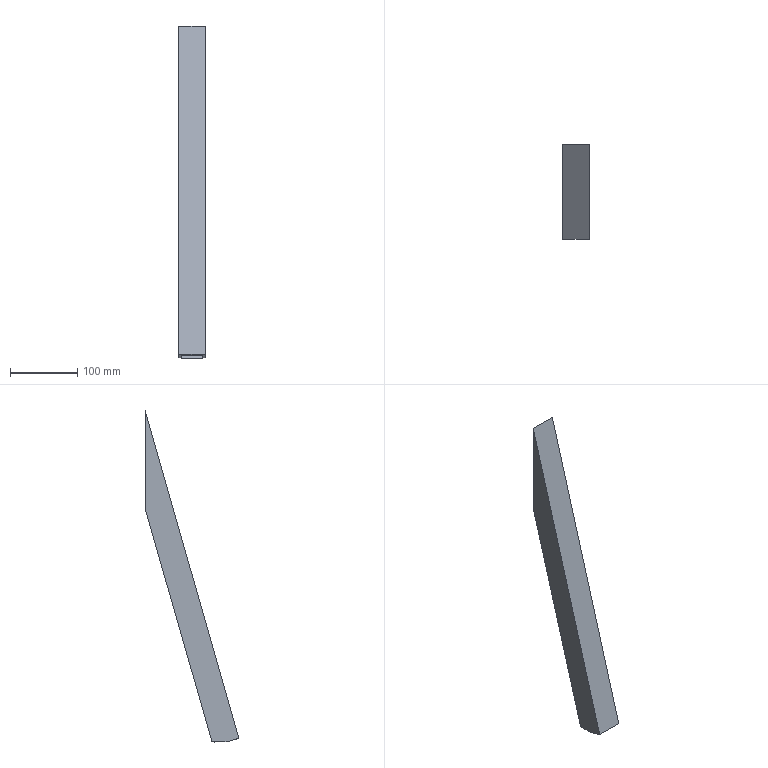Part | SolidWorks | features BaseBody 1 | 1 solid | 11 faces | box 40 x 139.228 x 491.982 mm | volume 250092 mm3 | plane 11
STEP:
#1=CARTESIAN_POINT('',(-230.,-189.228,31.503));
#2=VERTEX_POINT('',#1);
#3=CARTESIAN_POINT('',(-230.,-50.,517.982));
#4=VERTEX_POINT('',#3);
#5=CARTESIAN_POINT('',(-230.,-189.228,31.503));
#6=DIRECTION('',(0.,0.2751,0.9614));
#7=VECTOR('',#6,1000.);
#8=LINE('',#5,#7);
#9=EDGE_CURVE('',#2,#4,#8,.T.);
#10=ORIENTED_EDGE('',*,*,#9,.F.);
#11=CARTESIAN_POINT('',(-190.,-189.228,31.503));
#12=VERTEX_POINT('',#11);
#13=CARTESIAN_POINT('',(-190.,-189.228,31.503));
#14=DIRECTION('',(-1.,0.,0.));
#15=VECTOR('',#14,1000.);
#16=LINE('',#13,#15);
#17=EDGE_CURVE('',#12,#2,#16,.T.);
#18=ORIENTED_EDGE('',*,*,#17,.F.);
#19=CARTESIAN_POINT('',(-190.,-50.,517.982));
#20=VERTEX_POINT('',#19);
#21=CARTESIAN_POINT('',(-190.,-189.228,31.503));
#22=DIRECTION('',(0.,-0.2751,-0.9614));
#23=VECTOR('',#22,1000.);
#24=LINE('',#21,#23);
#25=EDGE_CURVE('',#20,#12,#24,.T.);
#26=ORIENTED_EDGE('',*,*,#25,.F.);
#27=CARTESIAN_POINT('',(-190.,-50.,517.982));
#28=DIRECTION('',(1.,0.,0.));
#29=VECTOR('',#28,1000.);
#30=LINE('',#27,#29);
#31=EDGE_CURVE('',#4,#20,#30,.T.);
#32=ORIENTED_EDGE('',*,*,#31,.F.);
#33=EDGE_LOOP('',(#10,#18,#26,#32));
#34=FACE_OUTER_BOUND('',#33,.T.);
#35=CARTESIAN_POINT('',(-190.,-189.228,31.503));
#36=DIRECTION('',(0.,0.9614,-0.2751));
#37=DIRECTION('',(0.,0.2751,0.9614));
#38=AXIS2_PLACEMENT_3D('',#35,#36,#37);
#39=PLANE('',#38);
#40=ADVANCED_FACE('',(#34),#39,.F.);
#41=CARTESIAN_POINT('',(-226.,-50.,503.445));
#42=VERTEX_POINT('',#41);
#43=CARTESIAN_POINT('',(-226.,-50.,387.144));
#44=VERTEX_POINT('',#43);
#45=CARTESIAN_POINT('',(-226.,-50.,28.));
#46=DIRECTION('',(0.,0.,-1.));
#47=VECTOR('',#46,1000.);
#48=LINE('',#45,#47);
#49=EDGE_CURVE('',#42,#44,#48,.T.);
#50=ORIENTED_EDGE('',*,*,#49,.T.);
#51=CARTESIAN_POINT('',(-194.,-50.,387.144));
#52=VERTEX_POINT('',#51);
#53=CARTESIAN_POINT('',(-260.,-50.,387.144));
#54=DIRECTION('',(1.,0.,0.));
#55=VECTOR('',#54,1000.);
#56=LINE('',#53,#55);
#57=EDGE_CURVE('',#44,#52,#56,.T.);
#58=ORIENTED_EDGE('',*,*,#57,.T.);
#59=CARTESIAN_POINT('',(-194.,-50.,503.445));
#60=VERTEX_POINT('',#59);
#61=CARTESIAN_POINT('',(-194.,-50.,28.));
#62=DIRECTION('',(0.,0.,1.));
#63=VECTOR('',#62,1000.);
#64=LINE('',#61,#63);
#65=EDGE_CURVE('',#52,#60,#64,.T.);
#66=ORIENTED_EDGE('',*,*,#65,.T.);
#67=CARTESIAN_POINT('',(-260.,-50.,503.445));
#68=DIRECTION('',(-1.,0.,0.));
#69=VECTOR('',#68,1000.);
#70=LINE('',#67,#69);
#71=EDGE_CURVE('',#60,#42,#70,.T.);
#72=ORIENTED_EDGE('',*,*,#71,.T.);
#73=EDGE_LOOP('',(#50,#58,#66,#72));
#74=FACE_BOUND('',#73,.T.);
#75=CARTESIAN_POINT('',(-190.,-50.,372.606));
#76=VERTEX_POINT('',#75);
#77=CARTESIAN_POINT('',(-190.,-50.,28.));
#78=DIRECTION('',(0.,0.,-1.));
#79=VECTOR('',#78,1000.);
#80=LINE('',#77,#79);
#81=EDGE_CURVE('',#20,#76,#80,.T.);
#82=ORIENTED_EDGE('',*,*,#81,.T.);
#83=CARTESIAN_POINT('',(-230.,-50.,372.606));
#84=VERTEX_POINT('',#83);
#85=CARTESIAN_POINT('',(-260.,-50.,372.606));
#86=DIRECTION('',(-1.,0.,0.));
#87=VECTOR('',#86,1000.);
#88=LINE('',#85,#87);
#89=EDGE_CURVE('',#76,#84,#88,.T.);
#90=ORIENTED_EDGE('',*,*,#89,.T.);
#91=CARTESIAN_POINT('',(-230.,-50.,28.));
#92=DIRECTION('',(0.,0.,1.));
#93=VECTOR('',#92,1000.);
#94=LINE('',#91,#93);
#95=EDGE_CURVE('',#84,#4,#94,.T.);
#96=ORIENTED_EDGE('',*,*,#95,.T.);
#97=ORIENTED_EDGE('',*,*,#31,.T.);
#98=EDGE_LOOP('',(#82,#90,#96,#97));
#99=FACE_OUTER_BOUND('',#98,.T.);
#100=CARTESIAN_POINT('',(-260.,-50.,28.));
#101=DIRECTION('',(0.,1.,0.));
#102=DIRECTION('',(0.,0.,1.));
#103=AXIS2_PLACEMENT_3D('',#100,#101,#102);
#104=PLANE('',#103);
#105=ADVANCED_FACE('',(#74,#99),#104,.T.);
#106=ORIENTED_EDGE('',*,*,#9,.T.);
#107=ORIENTED_EDGE('',*,*,#95,.F.);
#108=CARTESIAN_POINT('',(-230.,-149.197,26.));
#109=VERTEX_POINT('',#108);
#110=CARTESIAN_POINT('',(-230.,-50.,372.606));
#111=DIRECTION('',(0.,-0.2751,-0.9614));
#112=VECTOR('',#111,1000.);
#113=LINE('',#110,#112);
#114=EDGE_CURVE('',#84,#109,#113,.T.);
#115=ORIENTED_EDGE('',*,*,#114,.T.);
#116=CARTESIAN_POINT('',(-230.,-170.,26.));
#117=VERTEX_POINT('',#116);
#118=CARTESIAN_POINT('',(-230.,-189.228,26.));
#119=DIRECTION('',(0.,-1.,0.));
#120=VECTOR('',#119,1000.);
#121=LINE('',#118,#120);
#122=EDGE_CURVE('',#109,#117,#121,.T.);
#123=ORIENTED_EDGE('',*,*,#122,.T.);
#124=CARTESIAN_POINT('',(-230.,-170.,26.));
#125=DIRECTION('',(0.,-0.9614,0.2751));
#126=VECTOR('',#125,1000.);
#127=LINE('',#124,#126);
#128=EDGE_CURVE('',#117,#2,#127,.T.);
#129=ORIENTED_EDGE('',*,*,#128,.T.);
#130=EDGE_LOOP('',(#106,#107,#115,#123,#129));
#131=FACE_OUTER_BOUND('',#130,.T.);
#132=CARTESIAN_POINT('',(-230.,-189.228,31.503));
#133=DIRECTION('',(-1.,0.,0.));
#134=DIRECTION('',(0.,0.,1.));
#135=AXIS2_PLACEMENT_3D('',#132,#133,#134);
#136=PLANE('',#135);
#137=ADVANCED_FACE('',(#131),#136,.T.);
#138=CARTESIAN_POINT('',(-226.,-185.382,30.402));
#139=VERTEX_POINT('',#138);
#140=CARTESIAN_POINT('',(-226.,-170.,26.));
#141=VERTEX_POINT('',#140);
#142=CARTESIAN_POINT('',(-226.,-189.228,31.503));
#143=DIRECTION('',(0.,0.9614,-0.2751));
#144=VECTOR('',#143,1000.);
#145=LINE('',#142,#144);
#146=EDGE_CURVE('',#139,#141,#145,.T.);
#147=ORIENTED_EDGE('',*,*,#146,.F.);
#148=CARTESIAN_POINT('',(-194.,-185.382,30.402));
#149=VERTEX_POINT('',#148);
#150=CARTESIAN_POINT('',(-190.,-185.382,30.402));
#151=DIRECTION('',(-1.,0.,0.));
#152=VECTOR('',#151,1000.);
#153=LINE('',#150,#152);
#154=EDGE_CURVE('',#149,#139,#153,.T.);
#155=ORIENTED_EDGE('',*,*,#154,.F.);
#156=CARTESIAN_POINT('',(-194.,-170.,26.));
#157=VERTEX_POINT('',#156);
#158=CARTESIAN_POINT('',(-194.,-189.228,31.503));
#159=DIRECTION('',(0.,-0.9614,0.2751));
#160=VECTOR('',#159,1000.);
#161=LINE('',#158,#160);
#162=EDGE_CURVE('',#157,#149,#161,.T.);
#163=ORIENTED_EDGE('',*,*,#162,.F.);
#164=CARTESIAN_POINT('',(-190.,-170.,26.));
#165=VERTEX_POINT('',#164);
#166=CARTESIAN_POINT('',(-190.,-170.,26.));
#167=DIRECTION('',(-1.,0.,0.));
#168=VECTOR('',#167,1000.);
#169=LINE('',#166,#168);
#170=EDGE_CURVE('',#165,#157,#169,.T.);
#171=ORIENTED_EDGE('',*,*,#170,.F.);
#172=CARTESIAN_POINT('',(-190.,-189.228,31.503));
#173=DIRECTION('',(0.,0.9614,-0.2751));
#174=VECTOR('',#173,1000.);
#175=LINE('',#172,#174);
#176=EDGE_CURVE('',#12,#165,#175,.T.);
#177=ORIENTED_EDGE('',*,*,#176,.F.);
#178=ORIENTED_EDGE('',*,*,#17,.T.);
#179=ORIENTED_EDGE('',*,*,#128,.F.);
#180=CARTESIAN_POINT('',(-190.,-170.,26.));
#181=DIRECTION('',(-1.,0.,0.));
#182=VECTOR('',#181,1000.);
#183=LINE('',#180,#182);
#184=EDGE_CURVE('',#141,#117,#183,.T.);
#185=ORIENTED_EDGE('',*,*,#184,.F.);
#186=EDGE_LOOP('',(#147,#155,#163,#171,#177,#178,#179,#185));
#187=FACE_OUTER_BOUND('',#186,.T.);
#188=CARTESIAN_POINT('',(-190.,-189.228,31.503));
#189=DIRECTION('',(0.,0.2751,0.9614));
#190=DIRECTION('',(0.,-0.9614,0.2751));
#191=AXIS2_PLACEMENT_3D('',#188,#189,#190);
#192=PLANE('',#191);
#193=ADVANCED_FACE('',(#187),#192,.F.);
#194=ORIENTED_EDGE('',*,*,#25,.T.);
#195=ORIENTED_EDGE('',*,*,#176,.T.);
#196=CARTESIAN_POINT('',(-190.,-149.197,26.));
#197=VERTEX_POINT('',#196);
#198=CARTESIAN_POINT('',(-190.,-189.228,26.));
#199=DIRECTION('',(0.,-1.,0.));
#200=VECTOR('',#199,1000.);
#201=LINE('',#198,#200);
#202=EDGE_CURVE('',#197,#165,#201,.T.);
#203=ORIENTED_EDGE('',*,*,#202,.F.);
#204=CARTESIAN_POINT('',(-190.,-50.,372.606));
#205=DIRECTION('',(0.,-0.2751,-0.9614));
#206=VECTOR('',#205,1000.);
#207=LINE('',#204,#206);
#208=EDGE_CURVE('',#76,#197,#207,.T.);
#209=ORIENTED_EDGE('',*,*,#208,.F.);
#210=ORIENTED_EDGE('',*,*,#81,.F.);
#211=EDGE_LOOP('',(#194,#195,#203,#209,#210));
#212=FACE_OUTER_BOUND('',#211,.T.);
#213=CARTESIAN_POINT('',(-190.,-189.228,31.503));
#214=DIRECTION('',(-1.,0.,0.));
#215=DIRECTION('',(0.,0.,1.));
#216=AXIS2_PLACEMENT_3D('',#213,#214,#215);
#217=PLANE('',#216);
#218=ADVANCED_FACE('',(#212),#217,.F.);
#219=CARTESIAN_POINT('',(-226.,-153.358,26.));
#220=VERTEX_POINT('',#219);
#221=CARTESIAN_POINT('',(-226.,-154.893,20.636));
#222=DIRECTION('',(0.,0.2751,0.9614));
#223=VECTOR('',#222,1000.);
#224=LINE('',#221,#223);
#225=EDGE_CURVE('',#220,#44,#224,.T.);
#226=ORIENTED_EDGE('',*,*,#225,.F.);
#227=CARTESIAN_POINT('',(-194.,-153.358,26.));
#228=VERTEX_POINT('',#227);
#229=CARTESIAN_POINT('',(-194.,-153.358,26.));
#230=DIRECTION('',(-1.,0.,0.));
#231=VECTOR('',#230,1000.);
#232=LINE('',#229,#231);
#233=EDGE_CURVE('',#228,#220,#232,.T.);
#234=ORIENTED_EDGE('',*,*,#233,.F.);
#235=CARTESIAN_POINT('',(-194.,-154.893,20.636));
#236=DIRECTION('',(0.,-0.2751,-0.9614));
#237=VECTOR('',#236,1000.);
#238=LINE('',#235,#237);
#239=EDGE_CURVE('',#52,#228,#238,.T.);
#240=ORIENTED_EDGE('',*,*,#239,.F.);
#241=ORIENTED_EDGE('',*,*,#57,.F.);
#242=EDGE_LOOP('',(#226,#234,#240,#241));
#243=FACE_OUTER_BOUND('',#242,.T.);
#244=CARTESIAN_POINT('',(-194.,-154.893,20.636));
#245=DIRECTION('',(0.,0.9614,-0.2751));
#246=DIRECTION('',(0.,0.2751,0.9614));
#247=AXIS2_PLACEMENT_3D('',#244,#245,#246);
#248=PLANE('',#247);
#249=ADVANCED_FACE('',(#243),#248,.F.);
#250=CARTESIAN_POINT('',(-226.,-185.382,30.402));
#251=DIRECTION('',(0.,0.2751,0.9614));
#252=VECTOR('',#251,1000.);
#253=LINE('',#250,#252);
#254=EDGE_CURVE('',#139,#42,#253,.T.);
#255=ORIENTED_EDGE('',*,*,#254,.F.);
#256=ORIENTED_EDGE('',*,*,#146,.T.);
#257=CARTESIAN_POINT('',(-226.,-185.658,26.));
#258=DIRECTION('',(0.,-1.,0.));
#259=VECTOR('',#258,1000.);
#260=LINE('',#257,#259);
#261=EDGE_CURVE('',#220,#141,#260,.T.);
#262=ORIENTED_EDGE('',*,*,#261,.F.);
#263=ORIENTED_EDGE('',*,*,#225,.T.);
#264=ORIENTED_EDGE('',*,*,#49,.F.);
#265=EDGE_LOOP('',(#255,#256,#262,#263,#264));
#266=FACE_OUTER_BOUND('',#265,.T.);
#267=CARTESIAN_POINT('',(-226.,-185.658,29.441));
#268=DIRECTION('',(-1.,0.,0.));
#269=DIRECTION('',(0.,0.,1.));
#270=AXIS2_PLACEMENT_3D('',#267,#268,#269);
#271=PLANE('',#270);
#272=ADVANCED_FACE('',(#266),#271,.F.);
#273=ORIENTED_EDGE('',*,*,#254,.T.);
#274=ORIENTED_EDGE('',*,*,#71,.F.);
#275=CARTESIAN_POINT('',(-194.,-185.658,29.441));
#276=DIRECTION('',(0.,-0.2751,-0.9614));
#277=VECTOR('',#276,1000.);
#278=LINE('',#275,#277);
#279=EDGE_CURVE('',#60,#149,#278,.T.);
#280=ORIENTED_EDGE('',*,*,#279,.T.);
#281=ORIENTED_EDGE('',*,*,#154,.T.);
#282=EDGE_LOOP('',(#273,#274,#280,#281));
#283=FACE_OUTER_BOUND('',#282,.T.);
#284=CARTESIAN_POINT('',(-194.,-185.658,29.441));
#285=DIRECTION('',(0.,0.9614,-0.2751));
#286=DIRECTION('',(0.,0.2751,0.9614));
#287=AXIS2_PLACEMENT_3D('',#284,#285,#286);
#288=PLANE('',#287);
#289=ADVANCED_FACE('',(#283),#288,.T.);
#290=ORIENTED_EDGE('',*,*,#279,.F.);
#291=ORIENTED_EDGE('',*,*,#65,.F.);
#292=ORIENTED_EDGE('',*,*,#239,.T.);
#293=CARTESIAN_POINT('',(-194.,-185.658,26.));
#294=DIRECTION('',(0.,-1.,0.));
#295=VECTOR('',#294,1000.);
#296=LINE('',#293,#295);
#297=EDGE_CURVE('',#228,#157,#296,.T.);
#298=ORIENTED_EDGE('',*,*,#297,.T.);
#299=ORIENTED_EDGE('',*,*,#162,.T.);
#300=EDGE_LOOP('',(#290,#291,#292,#298,#299));
#301=FACE_OUTER_BOUND('',#300,.T.);
#302=CARTESIAN_POINT('',(-194.,-185.658,29.441));
#303=DIRECTION('',(-1.,0.,0.));
#304=DIRECTION('',(0.,0.,1.));
#305=AXIS2_PLACEMENT_3D('',#302,#303,#304);
#306=PLANE('',#305);
#307=ADVANCED_FACE('',(#301),#306,.T.);
#308=ORIENTED_EDGE('',*,*,#114,.F.);
#309=ORIENTED_EDGE('',*,*,#89,.F.);
#310=ORIENTED_EDGE('',*,*,#208,.T.);
#311=CARTESIAN_POINT('',(-190.,-149.197,26.));
#312=DIRECTION('',(-1.,0.,0.));
#313=VECTOR('',#312,1000.);
#314=LINE('',#311,#313);
#315=EDGE_CURVE('',#197,#109,#314,.T.);
#316=ORIENTED_EDGE('',*,*,#315,.T.);
#317=EDGE_LOOP('',(#308,#309,#310,#316));
#318=FACE_OUTER_BOUND('',#317,.T.);
#319=CARTESIAN_POINT('',(-190.,-150.772,20.497));
#320=DIRECTION('',(0.,0.9614,-0.2751));
#321=DIRECTION('',(0.,0.2751,0.9614));
#322=AXIS2_PLACEMENT_3D('',#319,#320,#321);
#323=PLANE('',#322);
#324=ADVANCED_FACE('',(#318),#323,.T.);
#325=ORIENTED_EDGE('',*,*,#233,.T.);
#326=ORIENTED_EDGE('',*,*,#261,.T.);
#327=ORIENTED_EDGE('',*,*,#184,.T.);
#328=ORIENTED_EDGE('',*,*,#122,.F.);
#329=ORIENTED_EDGE('',*,*,#315,.F.);
#330=ORIENTED_EDGE('',*,*,#202,.T.);
#331=ORIENTED_EDGE('',*,*,#170,.T.);
#332=ORIENTED_EDGE('',*,*,#297,.F.);
#333=EDGE_LOOP('',(#325,#326,#327,#328,#329,#330,#331,#332));
#334=FACE_OUTER_BOUND('',#333,.T.);
#335=CARTESIAN_POINT('',(-300.,-250.,26.));
#336=DIRECTION('',(0.,0.,1.));
#337=DIRECTION('',(1.,0.,0.));
#338=AXIS2_PLACEMENT_3D('',#335,#336,#337);
#339=PLANE('',#338);
#340=ADVANCED_FACE('',(#334),#339,.F.);
#341=CLOSED_SHELL('',(#40,#105,#137,#193,#218,#249,#272,#289,#307,#324,#340));
#342=MANIFOLD_SOLID_BREP('',#341);
#343=CARTESIAN_POINT('',(0.,0.,0.));
#344=DIRECTION('',(0.,0.,1.));
#345=DIRECTION('',(1.,0.,0.));
#346=AXIS2_PLACEMENT_3D('',#343,#344,#345);
#347=(LENGTH_UNIT()NAMED_UNIT(*)SI_UNIT(.MILLI.,.METRE.));
#348=UNCERTAINTY_MEASURE_WITH_UNIT(LENGTH_MEASURE(0.00001),#347,'','');
#349=(NAMED_UNIT(*)PLANE_ANGLE_UNIT()SI_UNIT($,.RADIAN.));
#350=(NAMED_UNIT(*)SI_UNIT($,.STERADIAN.)SOLID_ANGLE_UNIT());
#351=(GEOMETRIC_REPRESENTATION_CONTEXT(3)GLOBAL_UNCERTAINTY_ASSIGNED_CONTEXT((#348))GLOBAL_UNIT_ASSIGNED_CONTEXT((#347,#349,#350))REPRESENTATION_CONTEXT('',''));
#352=ADVANCED_BREP_SHAPE_REPRESENTATION('',(#342,#346),#351);